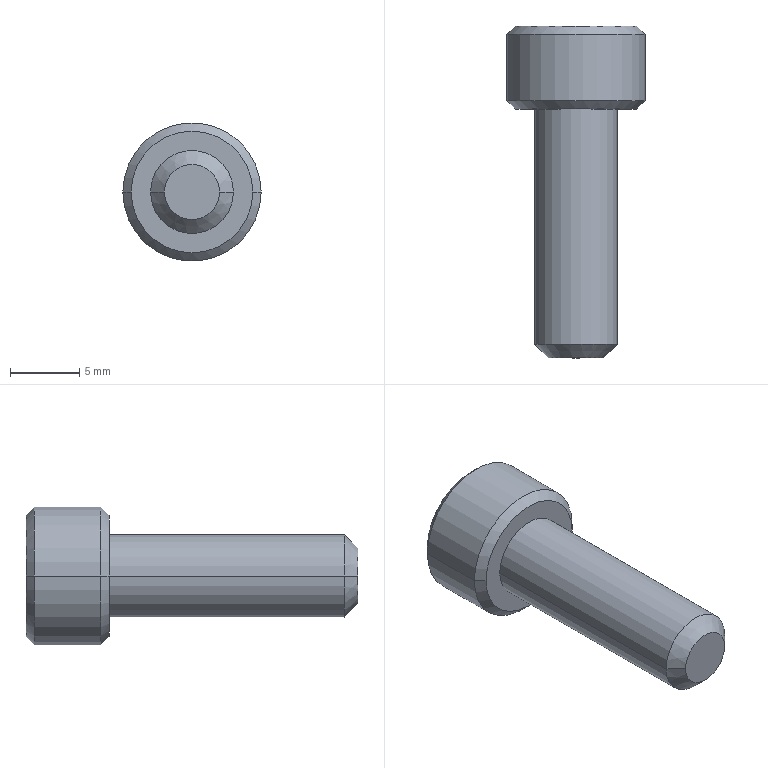Part | STEP file | BB62-M6-18L-6 | 1 solid | 27 faces | box 10 x 24 x 10 mm | volume 883.045 mm3 | plane 15 | cone 8 | cylinder 4 | commonest cylinder face diameters 6 x2 10 x2
STEP:
#1=CARTESIAN_POINT('',(0.,1.349,0.));
#2=VERTEX_POINT('',#1);
#3=CARTESIAN_POINT('',(2.86,3.,0.));
#4=VERTEX_POINT('',#3);
#5=CARTESIAN_POINT('',(0.,1.349,0.));
#6=DIRECTION('',(0.866,0.5,0.));
#7=VECTOR('',#6,1000.);
#8=LINE('',#5,#7);
#9=EDGE_CURVE('',#2,#4,#8,.T.);
#10=ORIENTED_EDGE('',*,*,#9,.F.);
#11=CARTESIAN_POINT('',(-2.86,3.,0.));
#12=VERTEX_POINT('',#11);
#13=CARTESIAN_POINT('',(0.,1.349,0.));
#14=DIRECTION('',(-0.866,0.5,0.));
#15=VECTOR('',#14,1000.);
#16=LINE('',#13,#15);
#17=EDGE_CURVE('',#2,#12,#16,.T.);
#18=ORIENTED_EDGE('',*,*,#17,.T.);
#19=CARTESIAN_POINT('',(-2.477,3.,1.43));
#20=VERTEX_POINT('',#19);
#21=CARTESIAN_POINT('',(0.,3.,0.));
#22=DIRECTION('',(0.,-1.,0.));
#23=DIRECTION('',(-1.,0.,0.));
#24=AXIS2_PLACEMENT_3D('',#21,#22,#23);
#25=CIRCLE('',#24,2.86);
#26=EDGE_CURVE('',#20,#12,#25,.T.);
#27=ORIENTED_EDGE('',*,*,#26,.F.);
#28=CARTESIAN_POINT('',(0.,3.,2.86));
#29=VERTEX_POINT('',#28);
#30=CARTESIAN_POINT('',(0.,3.,0.));
#31=DIRECTION('',(0.,-1.,0.));
#32=DIRECTION('',(-1.,0.,0.));
#33=AXIS2_PLACEMENT_3D('',#30,#31,#32);
#34=CIRCLE('',#33,2.86);
#35=EDGE_CURVE('',#29,#20,#34,.T.);
#36=ORIENTED_EDGE('',*,*,#35,.F.);
#37=CARTESIAN_POINT('',(2.477,3.,1.43));
#38=VERTEX_POINT('',#37);
#39=CARTESIAN_POINT('',(0.,3.,0.));
#40=DIRECTION('',(0.,-1.,0.));
#41=DIRECTION('',(-1.,0.,0.));
#42=AXIS2_PLACEMENT_3D('',#39,#40,#41);
#43=CIRCLE('',#42,2.86);
#44=EDGE_CURVE('',#38,#29,#43,.T.);
#45=ORIENTED_EDGE('',*,*,#44,.F.);
#46=CARTESIAN_POINT('',(0.,3.,0.));
#47=DIRECTION('',(0.,-1.,0.));
#48=DIRECTION('',(-1.,0.,0.));
#49=AXIS2_PLACEMENT_3D('',#46,#47,#48);
#50=CIRCLE('',#49,2.86);
#51=EDGE_CURVE('',#4,#38,#50,.T.);
#52=ORIENTED_EDGE('',*,*,#51,.F.);
#53=EDGE_LOOP('',(#10,#18,#27,#36,#45,#52));
#54=FACE_OUTER_BOUND('',#53,.T.);
#55=CARTESIAN_POINT('',(0.,1001.349,0.));
#56=DIRECTION('',(0.,1.,0.));
#57=DIRECTION('',(1.,0.,0.));
#58=AXIS2_PLACEMENT_3D('',#55,#56,#57);
#59=CONICAL_SURFACE('',#58,1732.051,1.047);
#60=ADVANCED_FACE('',(#54),#59,.F.);
#61=CARTESIAN_POINT('',(2.,-18.,0.));
#62=VERTEX_POINT('',#61);
#63=CARTESIAN_POINT('',(-2.,-18.,0.));
#64=VERTEX_POINT('',#63);
#65=CARTESIAN_POINT('',(0.,-18.,0.));
#66=DIRECTION('',(0.,1.,0.));
#67=DIRECTION('',(1.,0.,0.));
#68=AXIS2_PLACEMENT_3D('',#65,#66,#67);
#69=CIRCLE('',#68,2.);
#70=EDGE_CURVE('',#62,#64,#69,.T.);
#71=ORIENTED_EDGE('',*,*,#70,.T.);
#72=CARTESIAN_POINT('',(-3.,-17.,0.));
#73=VERTEX_POINT('',#72);
#74=CARTESIAN_POINT('',(-2.,-18.,0.));
#75=DIRECTION('',(-0.7071,0.7071,0.));
#76=VECTOR('',#75,1000.);
#77=LINE('',#74,#76);
#78=EDGE_CURVE('',#64,#73,#77,.T.);
#79=ORIENTED_EDGE('',*,*,#78,.T.);
#80=CARTESIAN_POINT('',(3.,-17.,0.));
#81=VERTEX_POINT('',#80);
#82=CARTESIAN_POINT('',(0.,-17.,0.));
#83=DIRECTION('',(0.,-1.,0.));
#84=DIRECTION('',(-1.,0.,0.));
#85=AXIS2_PLACEMENT_3D('',#82,#83,#84);
#86=CIRCLE('',#85,3.);
#87=EDGE_CURVE('',#73,#81,#86,.T.);
#88=ORIENTED_EDGE('',*,*,#87,.T.);
#89=CARTESIAN_POINT('',(2.,-18.,0.));
#90=DIRECTION('',(0.7071,0.7071,0.));
#91=VECTOR('',#90,1000.);
#92=LINE('',#89,#91);
#93=EDGE_CURVE('',#62,#81,#92,.T.);
#94=ORIENTED_EDGE('',*,*,#93,.F.);
#95=EDGE_LOOP('',(#71,#79,#88,#94));
#96=FACE_OUTER_BOUND('',#95,.T.);
#97=CARTESIAN_POINT('',(0.,-18.,0.));
#98=DIRECTION('',(0.,1.,0.));
#99=DIRECTION('',(1.,0.,0.));
#100=AXIS2_PLACEMENT_3D('',#97,#98,#99);
#101=CONICAL_SURFACE('',#100,2.,0.7854);
#102=ADVANCED_FACE('',(#96),#101,.T.);
#103=ORIENTED_EDGE('',*,*,#87,.F.);
#104=CARTESIAN_POINT('',(-3.,0.,0.));
#105=VERTEX_POINT('',#104);
#106=CARTESIAN_POINT('',(-3.,-17.,0.));
#107=DIRECTION('',(0.,1.,0.));
#108=VECTOR('',#107,1000.);
#109=LINE('',#106,#108);
#110=EDGE_CURVE('',#73,#105,#109,.T.);
#111=ORIENTED_EDGE('',*,*,#110,.T.);
#112=CARTESIAN_POINT('',(3.,0.,0.));
#113=VERTEX_POINT('',#112);
#114=CARTESIAN_POINT('',(0.,0.,0.));
#115=DIRECTION('',(0.,-1.,0.));
#116=DIRECTION('',(-1.,0.,0.));
#117=AXIS2_PLACEMENT_3D('',#114,#115,#116);
#118=CIRCLE('',#117,3.);
#119=EDGE_CURVE('',#105,#113,#118,.T.);
#120=ORIENTED_EDGE('',*,*,#119,.T.);
#121=CARTESIAN_POINT('',(3.,-17.,0.));
#122=DIRECTION('',(0.,1.,0.));
#123=VECTOR('',#122,1000.);
#124=LINE('',#121,#123);
#125=EDGE_CURVE('',#81,#113,#124,.T.);
#126=ORIENTED_EDGE('',*,*,#125,.F.);
#127=EDGE_LOOP('',(#103,#111,#120,#126));
#128=FACE_OUTER_BOUND('',#127,.T.);
#129=CARTESIAN_POINT('',(0.,-17.,0.));
#130=DIRECTION('',(0.,1.,0.));
#131=DIRECTION('',(1.,0.,0.));
#132=AXIS2_PLACEMENT_3D('',#129,#130,#131);
#133=CYLINDRICAL_SURFACE('',#132,3.);
#134=ADVANCED_FACE('',(#128),#133,.T.);
#135=CARTESIAN_POINT('',(-4.4,6.,0.));
#136=VERTEX_POINT('',#135);
#137=CARTESIAN_POINT('',(4.4,6.,0.));
#138=VERTEX_POINT('',#137);
#139=CARTESIAN_POINT('',(0.,6.,0.));
#140=DIRECTION('',(0.,-1.,0.));
#141=DIRECTION('',(-1.,0.,0.));
#142=AXIS2_PLACEMENT_3D('',#139,#140,#141);
#143=CIRCLE('',#142,4.4);
#144=EDGE_CURVE('',#136,#138,#143,.T.);
#145=ORIENTED_EDGE('',*,*,#144,.T.);
#146=CARTESIAN_POINT('',(5.,5.4,0.));
#147=VERTEX_POINT('',#146);
#148=CARTESIAN_POINT('',(5.,5.4,0.));
#149=DIRECTION('',(0.7071,-0.7071,0.));
#150=VECTOR('',#149,1000.);
#151=LINE('',#148,#150);
#152=EDGE_CURVE('',#138,#147,#151,.T.);
#153=ORIENTED_EDGE('',*,*,#152,.T.);
#154=CARTESIAN_POINT('',(-5.,5.4,0.));
#155=VERTEX_POINT('',#154);
#156=CARTESIAN_POINT('',(0.,5.4,0.));
#157=DIRECTION('',(0.,-1.,0.));
#158=DIRECTION('',(-1.,0.,0.));
#159=AXIS2_PLACEMENT_3D('',#156,#157,#158);
#160=CIRCLE('',#159,5.);
#161=EDGE_CURVE('',#155,#147,#160,.T.);
#162=ORIENTED_EDGE('',*,*,#161,.F.);
#163=CARTESIAN_POINT('',(-5.,5.4,0.));
#164=DIRECTION('',(-0.7071,-0.7071,0.));
#165=VECTOR('',#164,1000.);
#166=LINE('',#163,#165);
#167=EDGE_CURVE('',#136,#155,#166,.T.);
#168=ORIENTED_EDGE('',*,*,#167,.F.);
#169=EDGE_LOOP('',(#145,#153,#162,#168));
#170=FACE_OUTER_BOUND('',#169,.T.);
#171=CARTESIAN_POINT('',(0.,5.4,0.));
#172=DIRECTION('',(0.,-1.,0.));
#173=DIRECTION('',(-1.,0.,0.));
#174=AXIS2_PLACEMENT_3D('',#171,#172,#173);
#175=CONICAL_SURFACE('',#174,5.,0.7854);
#176=ADVANCED_FACE('',(#170),#175,.T.);
#177=ORIENTED_EDGE('',*,*,#161,.T.);
#178=CARTESIAN_POINT('',(5.,0.6,0.));
#179=VERTEX_POINT('',#178);
#180=CARTESIAN_POINT('',(5.,1.62,0.));
#181=DIRECTION('',(0.,-1.,0.));
#182=VECTOR('',#181,1000.);
#183=LINE('',#180,#182);
#184=EDGE_CURVE('',#147,#179,#183,.T.);
#185=ORIENTED_EDGE('',*,*,#184,.T.);
#186=CARTESIAN_POINT('',(-5.,0.6,0.));
#187=VERTEX_POINT('',#186);
#188=CARTESIAN_POINT('',(0.,0.6,0.));
#189=DIRECTION('',(0.,-1.,0.));
#190=DIRECTION('',(-1.,0.,0.));
#191=AXIS2_PLACEMENT_3D('',#188,#189,#190);
#192=CIRCLE('',#191,5.);
#193=EDGE_CURVE('',#187,#179,#192,.T.);
#194=ORIENTED_EDGE('',*,*,#193,.F.);
#195=CARTESIAN_POINT('',(-5.,1.62,0.));
#196=DIRECTION('',(0.,-1.,0.));
#197=VECTOR('',#196,1000.);
#198=LINE('',#195,#197);
#199=EDGE_CURVE('',#155,#187,#198,.T.);
#200=ORIENTED_EDGE('',*,*,#199,.F.);
#201=EDGE_LOOP('',(#177,#185,#194,#200));
#202=FACE_OUTER_BOUND('',#201,.T.);
#203=CARTESIAN_POINT('',(0.,1.62,0.));
#204=DIRECTION('',(0.,-1.,0.));
#205=DIRECTION('',(-1.,0.,0.));
#206=AXIS2_PLACEMENT_3D('',#203,#204,#205);
#207=CYLINDRICAL_SURFACE('',#206,5.);
#208=ADVANCED_FACE('',(#202),#207,.T.);
#209=CARTESIAN_POINT('',(-4.4,0.,0.));
#210=VERTEX_POINT('',#209);
#211=CARTESIAN_POINT('',(4.4,0.,0.));
#212=VERTEX_POINT('',#211);
#213=CARTESIAN_POINT('',(0.,0.,0.));
#214=DIRECTION('',(0.,-1.,0.));
#215=DIRECTION('',(-1.,0.,0.));
#216=AXIS2_PLACEMENT_3D('',#213,#214,#215);
#217=CIRCLE('',#216,4.4);
#218=EDGE_CURVE('',#210,#212,#217,.T.);
#219=ORIENTED_EDGE('',*,*,#218,.F.);
#220=CARTESIAN_POINT('',(-4.4,0.,0.));
#221=DIRECTION('',(-0.7071,0.7071,0.));
#222=VECTOR('',#221,1000.);
#223=LINE('',#220,#222);
#224=EDGE_CURVE('',#210,#187,#223,.T.);
#225=ORIENTED_EDGE('',*,*,#224,.T.);
#226=ORIENTED_EDGE('',*,*,#193,.T.);
#227=CARTESIAN_POINT('',(4.4,0.,0.));
#228=DIRECTION('',(0.7071,0.7071,0.));
#229=VECTOR('',#228,1000.);
#230=LINE('',#227,#229);
#231=EDGE_CURVE('',#212,#179,#230,.T.);
#232=ORIENTED_EDGE('',*,*,#231,.F.);
#233=EDGE_LOOP('',(#219,#225,#226,#232));
#234=FACE_OUTER_BOUND('',#233,.T.);
#235=CARTESIAN_POINT('',(0.,0.,0.));
#236=DIRECTION('',(0.,1.,0.));
#237=DIRECTION('',(1.,0.,0.));
#238=AXIS2_PLACEMENT_3D('',#235,#236,#237);
#239=CONICAL_SURFACE('',#238,4.4,0.7854);
#240=ADVANCED_FACE('',(#234),#239,.T.);
#241=ORIENTED_EDGE('',*,*,#144,.F.);
#242=CARTESIAN_POINT('',(0.,6.,0.));
#243=DIRECTION('',(0.,-1.,0.));
#244=DIRECTION('',(-1.,0.,0.));
#245=AXIS2_PLACEMENT_3D('',#242,#243,#244);
#246=CIRCLE('',#245,4.4);
#247=EDGE_CURVE('',#138,#136,#246,.T.);
#248=ORIENTED_EDGE('',*,*,#247,.F.);
#249=EDGE_LOOP('',(#241,#248));
#250=FACE_OUTER_BOUND('',#249,.T.);
#251=CARTESIAN_POINT('',(0.,6.,-2.86));
#252=VERTEX_POINT('',#251);
#253=CARTESIAN_POINT('',(-2.477,6.,-1.43));
#254=VERTEX_POINT('',#253);
#255=CARTESIAN_POINT('',(0.,6.,-2.86));
#256=DIRECTION('',(-0.866,0.,0.5));
#257=VECTOR('',#256,1000.);
#258=LINE('',#255,#257);
#259=EDGE_CURVE('',#252,#254,#258,.T.);
#260=ORIENTED_EDGE('',*,*,#259,.F.);
#261=CARTESIAN_POINT('',(2.477,6.,-1.43));
#262=VERTEX_POINT('',#261);
#263=CARTESIAN_POINT('',(2.477,6.,-1.43));
#264=DIRECTION('',(-0.866,0.,-0.5));
#265=VECTOR('',#264,1000.);
#266=LINE('',#263,#265);
#267=EDGE_CURVE('',#262,#252,#266,.T.);
#268=ORIENTED_EDGE('',*,*,#267,.F.);
#269=CARTESIAN_POINT('',(2.477,6.,1.43));
#270=VERTEX_POINT('',#269);
#271=CARTESIAN_POINT('',(2.477,6.,1.43));
#272=DIRECTION('',(0.,0.,-1.));
#273=VECTOR('',#272,1000.);
#274=LINE('',#271,#273);
#275=EDGE_CURVE('',#270,#262,#274,.T.);
#276=ORIENTED_EDGE('',*,*,#275,.F.);
#277=CARTESIAN_POINT('',(0.,6.,2.86));
#278=VERTEX_POINT('',#277);
#279=CARTESIAN_POINT('',(0.,6.,2.86));
#280=DIRECTION('',(0.866,0.,-0.5));
#281=VECTOR('',#280,1000.);
#282=LINE('',#279,#281);
#283=EDGE_CURVE('',#278,#270,#282,.T.);
#284=ORIENTED_EDGE('',*,*,#283,.F.);
#285=CARTESIAN_POINT('',(-2.477,6.,1.43));
#286=VERTEX_POINT('',#285);
#287=CARTESIAN_POINT('',(-2.477,6.,1.43));
#288=DIRECTION('',(0.866,0.,0.5));
#289=VECTOR('',#288,1000.);
#290=LINE('',#287,#289);
#291=EDGE_CURVE('',#286,#278,#290,.T.);
#292=ORIENTED_EDGE('',*,*,#291,.F.);
#293=CARTESIAN_POINT('',(-2.477,6.,-1.43));
#294=DIRECTION('',(0.,0.,1.));
#295=VECTOR('',#294,1000.);
#296=LINE('',#293,#295);
#297=EDGE_CURVE('',#254,#286,#296,.T.);
#298=ORIENTED_EDGE('',*,*,#297,.F.);
#299=EDGE_LOOP('',(#260,#268,#276,#284,#292,#298));
#300=FACE_BOUND('',#299,.T.);
#301=CARTESIAN_POINT('',(4.4,6.,0.));
#302=DIRECTION('',(0.,1.,0.));
#303=DIRECTION('',(1.,0.,0.));
#304=AXIS2_PLACEMENT_3D('',#301,#302,#303);
#305=PLANE('',#304);
#306=ADVANCED_FACE('',(#250,#300),#305,.T.);
#307=CARTESIAN_POINT('',(0.,0.,0.));
#308=DIRECTION('',(0.,-1.,0.));
#309=DIRECTION('',(-1.,0.,0.));
#310=AXIS2_PLACEMENT_3D('',#307,#308,#309);
#311=CIRCLE('',#310,3.);
#312=EDGE_CURVE('',#113,#105,#311,.T.);
#313=ORIENTED_EDGE('',*,*,#312,.F.);
#314=ORIENTED_EDGE('',*,*,#119,.F.);
#315=EDGE_LOOP('',(#313,#314));
#316=FACE_BOUND('',#315,.T.);
#317=CARTESIAN_POINT('',(0.,0.,0.));
#318=DIRECTION('',(0.,-1.,0.));
#319=DIRECTION('',(-1.,0.,0.));
#320=AXIS2_PLACEMENT_3D('',#317,#318,#319);
#321=CIRCLE('',#320,4.4);
#322=EDGE_CURVE('',#212,#210,#321,.T.);
#323=ORIENTED_EDGE('',*,*,#322,.T.);
#324=ORIENTED_EDGE('',*,*,#218,.T.);
#325=EDGE_LOOP('',(#323,#324));
#326=FACE_OUTER_BOUND('',#325,.T.);
#327=CARTESIAN_POINT('',(0.,0.,0.));
#328=DIRECTION('',(0.,-1.,0.));
#329=DIRECTION('',(-1.,0.,0.));
#330=AXIS2_PLACEMENT_3D('',#327,#328,#329);
#331=PLANE('',#330);
#332=ADVANCED_FACE('',(#316,#326),#331,.T.);
#333=ORIENTED_EDGE('',*,*,#224,.F.);
#334=ORIENTED_EDGE('',*,*,#322,.F.);
#335=ORIENTED_EDGE('',*,*,#231,.T.);
#336=CARTESIAN_POINT('',(0.,0.6,0.));
#337=DIRECTION('',(0.,-1.,0.));
#338=DIRECTION('',(-1.,0.,0.));
#339=AXIS2_PLACEMENT_3D('',#336,#337,#338);
#340=CIRCLE('',#339,5.);
#341=EDGE_CURVE('',#179,#187,#340,.T.);
#342=ORIENTED_EDGE('',*,*,#341,.T.);
#343=EDGE_LOOP('',(#333,#334,#335,#342));
#344=FACE_OUTER_BOUND('',#343,.T.);
#345=CARTESIAN_POINT('',(0.,0.,0.));
#346=DIRECTION('',(0.,1.,0.));
#347=DIRECTION('',(1.,0.,0.));
#348=AXIS2_PLACEMENT_3D('',#345,#346,#347);
#349=CONICAL_SURFACE('',#348,4.4,0.7854);
#350=ADVANCED_FACE('',(#344),#349,.T.);
#351=ORIENTED_EDGE('',*,*,#184,.F.);
#352=CARTESIAN_POINT('',(0.,5.4,0.));
#353=DIRECTION('',(0.,-1.,0.));
#354=DIRECTION('',(-1.,0.,0.));
#355=AXIS2_PLACEMENT_3D('',#352,#353,#354);
#356=CIRCLE('',#355,5.);
#357=EDGE_CURVE('',#147,#155,#356,.T.);
#358=ORIENTED_EDGE('',*,*,#357,.T.);
#359=ORIENTED_EDGE('',*,*,#199,.T.);
#360=ORIENTED_EDGE('',*,*,#341,.F.);
#361=EDGE_LOOP('',(#351,#358,#359,#360));
#362=FACE_OUTER_BOUND('',#361,.T.);
#363=CARTESIAN_POINT('',(0.,1.62,0.));
#364=DIRECTION('',(0.,-1.,0.));
#365=DIRECTION('',(-1.,0.,0.));
#366=AXIS2_PLACEMENT_3D('',#363,#364,#365);
#367=CYLINDRICAL_SURFACE('',#366,5.);
#368=ADVANCED_FACE('',(#362),#367,.T.);
#369=ORIENTED_EDGE('',*,*,#152,.F.);
#370=ORIENTED_EDGE('',*,*,#247,.T.);
#371=ORIENTED_EDGE('',*,*,#167,.T.);
#372=ORIENTED_EDGE('',*,*,#357,.F.);
#373=EDGE_LOOP('',(#369,#370,#371,#372));
#374=FACE_OUTER_BOUND('',#373,.T.);
#375=CARTESIAN_POINT('',(0.,5.4,0.));
#376=DIRECTION('',(0.,-1.,0.));
#377=DIRECTION('',(-1.,0.,0.));
#378=AXIS2_PLACEMENT_3D('',#375,#376,#377);
#379=CONICAL_SURFACE('',#378,5.,0.7854);
#380=ADVANCED_FACE('',(#374),#379,.T.);
#381=ORIENTED_EDGE('',*,*,#110,.F.);
#382=CARTESIAN_POINT('',(0.,-17.,0.));
#383=DIRECTION('',(0.,-1.,0.));
#384=DIRECTION('',(-1.,0.,0.));
#385=AXIS2_PLACEMENT_3D('',#382,#383,#384);
#386=CIRCLE('',#385,3.);
#387=EDGE_CURVE('',#81,#73,#386,.T.);
#388=ORIENTED_EDGE('',*,*,#387,.F.);
#389=ORIENTED_EDGE('',*,*,#125,.T.);
#390=ORIENTED_EDGE('',*,*,#312,.T.);
#391=EDGE_LOOP('',(#381,#388,#389,#390));
#392=FACE_OUTER_BOUND('',#391,.T.);
#393=CARTESIAN_POINT('',(0.,-17.,0.));
#394=DIRECTION('',(0.,1.,0.));
#395=DIRECTION('',(1.,0.,0.));
#396=AXIS2_PLACEMENT_3D('',#393,#394,#395);
#397=CYLINDRICAL_SURFACE('',#396,3.);
#398=ADVANCED_FACE('',(#392),#397,.T.);
#399=ORIENTED_EDGE('',*,*,#70,.F.);
#400=CARTESIAN_POINT('',(0.,-18.,0.));
#401=DIRECTION('',(0.,1.,0.));
#402=DIRECTION('',(1.,0.,0.));
#403=AXIS2_PLACEMENT_3D('',#400,#401,#402);
#404=CIRCLE('',#403,2.);
#405=EDGE_CURVE('',#64,#62,#404,.T.);
#406=ORIENTED_EDGE('',*,*,#405,.F.);
#407=EDGE_LOOP('',(#399,#406));
#408=FACE_OUTER_BOUND('',#407,.T.);
#409=CARTESIAN_POINT('',(0.,-18.,0.));
#410=DIRECTION('',(0.,-1.,0.));
#411=DIRECTION('',(-1.,0.,0.));
#412=AXIS2_PLACEMENT_3D('',#409,#410,#411);
#413=PLANE('',#412);
#414=ADVANCED_FACE('',(#408),#413,.T.);
#415=ORIENTED_EDGE('',*,*,#78,.F.);
#416=ORIENTED_EDGE('',*,*,#405,.T.);
#417=ORIENTED_EDGE('',*,*,#93,.T.);
#418=ORIENTED_EDGE('',*,*,#387,.T.);
#419=EDGE_LOOP('',(#415,#416,#417,#418));
#420=FACE_OUTER_BOUND('',#419,.T.);
#421=CARTESIAN_POINT('',(0.,-18.,0.));
#422=DIRECTION('',(0.,1.,0.));
#423=DIRECTION('',(1.,0.,0.));
#424=AXIS2_PLACEMENT_3D('',#421,#422,#423);
#425=CONICAL_SURFACE('',#424,2.,0.7854);
#426=ADVANCED_FACE('',(#420),#425,.T.);
#427=CARTESIAN_POINT('',(2.477,3.,-1.43));
#428=VERTEX_POINT('',#427);
#429=CARTESIAN_POINT('',(0.,3.,-2.86));
#430=VERTEX_POINT('',#429);
#431=CARTESIAN_POINT('',(2.477,3.,-1.43));
#432=DIRECTION('',(-0.866,0.,-0.5));
#433=VECTOR('',#432,1000.);
#434=LINE('',#431,#433);
#435=EDGE_CURVE('',#428,#430,#434,.T.);
#436=ORIENTED_EDGE('',*,*,#435,.F.);
#437=CARTESIAN_POINT('',(2.477,6.,-1.43));
#438=DIRECTION('',(0.,-1.,0.));
#439=VECTOR('',#438,1000.);
#440=LINE('',#437,#439);
#441=EDGE_CURVE('',#262,#428,#440,.T.);
#442=ORIENTED_EDGE('',*,*,#441,.F.);
#443=ORIENTED_EDGE('',*,*,#267,.T.);
#444=CARTESIAN_POINT('',(0.,6.,-2.86));
#445=DIRECTION('',(0.,-1.,0.));
#446=VECTOR('',#445,1000.);
#447=LINE('',#444,#446);
#448=EDGE_CURVE('',#252,#430,#447,.T.);
#449=ORIENTED_EDGE('',*,*,#448,.T.);
#450=EDGE_LOOP('',(#436,#442,#443,#449));
#451=FACE_OUTER_BOUND('',#450,.T.);
#452=CARTESIAN_POINT('',(2.477,6.,-1.43));
#453=DIRECTION('',(-0.5,0.,0.866));
#454=DIRECTION('',(0.866,0.,0.5));
#455=AXIS2_PLACEMENT_3D('',#452,#453,#454);
#456=PLANE('',#455);
#457=ADVANCED_FACE('',(#451),#456,.T.);
#458=CARTESIAN_POINT('',(-2.477,3.,-1.43));
#459=VERTEX_POINT('',#458);
#460=CARTESIAN_POINT('',(0.,3.,-2.86));
#461=DIRECTION('',(-0.866,0.,0.5));
#462=VECTOR('',#461,1000.);
#463=LINE('',#460,#462);
#464=EDGE_CURVE('',#430,#459,#463,.T.);
#465=ORIENTED_EDGE('',*,*,#464,.F.);
#466=ORIENTED_EDGE('',*,*,#448,.F.);
#467=ORIENTED_EDGE('',*,*,#259,.T.);
#468=CARTESIAN_POINT('',(-2.477,6.,-1.43));
#469=DIRECTION('',(0.,-1.,0.));
#470=VECTOR('',#469,1000.);
#471=LINE('',#468,#470);
#472=EDGE_CURVE('',#254,#459,#471,.T.);
#473=ORIENTED_EDGE('',*,*,#472,.T.);
#474=EDGE_LOOP('',(#465,#466,#467,#473));
#475=FACE_OUTER_BOUND('',#474,.T.);
#476=CARTESIAN_POINT('',(0.,6.,-2.86));
#477=DIRECTION('',(0.5,0.,0.866));
#478=DIRECTION('',(0.866,0.,-0.5));
#479=AXIS2_PLACEMENT_3D('',#476,#477,#478);
#480=PLANE('',#479);
#481=ADVANCED_FACE('',(#475),#480,.T.);
#482=CARTESIAN_POINT('',(-2.477,3.,-1.43));
#483=DIRECTION('',(0.,0.,1.));
#484=VECTOR('',#483,1000.);
#485=LINE('',#482,#484);
#486=EDGE_CURVE('',#459,#20,#485,.T.);
#487=ORIENTED_EDGE('',*,*,#486,.F.);
#488=ORIENTED_EDGE('',*,*,#472,.F.);
#489=ORIENTED_EDGE('',*,*,#297,.T.);
#490=CARTESIAN_POINT('',(-2.477,6.,1.43));
#491=DIRECTION('',(0.,-1.,0.));
#492=VECTOR('',#491,1000.);
#493=LINE('',#490,#492);
#494=EDGE_CURVE('',#286,#20,#493,.T.);
#495=ORIENTED_EDGE('',*,*,#494,.T.);
#496=EDGE_LOOP('',(#487,#488,#489,#495));
#497=FACE_OUTER_BOUND('',#496,.T.);
#498=CARTESIAN_POINT('',(-2.477,6.,-1.43));
#499=DIRECTION('',(1.,0.,0.));
#500=DIRECTION('',(0.,0.,-1.));
#501=AXIS2_PLACEMENT_3D('',#498,#499,#500);
#502=PLANE('',#501);
#503=ADVANCED_FACE('',(#497),#502,.T.);
#504=CARTESIAN_POINT('',(-2.477,3.,1.43));
#505=DIRECTION('',(0.866,0.,0.5));
#506=VECTOR('',#505,1000.);
#507=LINE('',#504,#506);
#508=EDGE_CURVE('',#20,#29,#507,.T.);
#509=ORIENTED_EDGE('',*,*,#508,.F.);
#510=ORIENTED_EDGE('',*,*,#494,.F.);
#511=ORIENTED_EDGE('',*,*,#291,.T.);
#512=CARTESIAN_POINT('',(0.,6.,2.86));
#513=DIRECTION('',(0.,-1.,0.));
#514=VECTOR('',#513,1000.);
#515=LINE('',#512,#514);
#516=EDGE_CURVE('',#278,#29,#515,.T.);
#517=ORIENTED_EDGE('',*,*,#516,.T.);
#518=EDGE_LOOP('',(#509,#510,#511,#517));
#519=FACE_OUTER_BOUND('',#518,.T.);
#520=CARTESIAN_POINT('',(-2.477,6.,1.43));
#521=DIRECTION('',(0.5,0.,-0.866));
#522=DIRECTION('',(-0.866,0.,-0.5));
#523=AXIS2_PLACEMENT_3D('',#520,#521,#522);
#524=PLANE('',#523);
#525=ADVANCED_FACE('',(#519),#524,.T.);
#526=CARTESIAN_POINT('',(0.,3.,2.86));
#527=DIRECTION('',(0.866,0.,-0.5));
#528=VECTOR('',#527,1000.);
#529=LINE('',#526,#528);
#530=EDGE_CURVE('',#29,#38,#529,.T.);
#531=ORIENTED_EDGE('',*,*,#530,.F.);
#532=ORIENTED_EDGE('',*,*,#516,.F.);
#533=ORIENTED_EDGE('',*,*,#283,.T.);
#534=CARTESIAN_POINT('',(2.477,6.,1.43));
#535=DIRECTION('',(0.,-1.,0.));
#536=VECTOR('',#535,1000.);
#537=LINE('',#534,#536);
#538=EDGE_CURVE('',#270,#38,#537,.T.);
#539=ORIENTED_EDGE('',*,*,#538,.T.);
#540=EDGE_LOOP('',(#531,#532,#533,#539));
#541=FACE_OUTER_BOUND('',#540,.T.);
#542=CARTESIAN_POINT('',(0.,6.,2.86));
#543=DIRECTION('',(-0.5,0.,-0.866));
#544=DIRECTION('',(-0.866,0.,0.5));
#545=AXIS2_PLACEMENT_3D('',#542,#543,#544);
#546=PLANE('',#545);
#547=ADVANCED_FACE('',(#541),#546,.T.);
#548=CARTESIAN_POINT('',(2.477,3.,1.43));
#549=DIRECTION('',(0.,0.,-1.));
#550=VECTOR('',#549,1000.);
#551=LINE('',#548,#550);
#552=EDGE_CURVE('',#38,#428,#551,.T.);
#553=ORIENTED_EDGE('',*,*,#552,.F.);
#554=ORIENTED_EDGE('',*,*,#538,.F.);
#555=ORIENTED_EDGE('',*,*,#275,.T.);
#556=ORIENTED_EDGE('',*,*,#441,.T.);
#557=EDGE_LOOP('',(#553,#554,#555,#556));
#558=FACE_OUTER_BOUND('',#557,.T.);
#559=CARTESIAN_POINT('',(2.477,6.,1.43));
#560=DIRECTION('',(-1.,0.,0.));
#561=DIRECTION('',(0.,0.,1.));
#562=AXIS2_PLACEMENT_3D('',#559,#560,#561);
#563=PLANE('',#562);
#564=ADVANCED_FACE('',(#558),#563,.T.);
#565=ORIENTED_EDGE('',*,*,#435,.T.);
#566=CARTESIAN_POINT('',(0.,3.,0.));
#567=DIRECTION('',(0.,-1.,0.));
#568=DIRECTION('',(-1.,0.,0.));
#569=AXIS2_PLACEMENT_3D('',#566,#567,#568);
#570=CIRCLE('',#569,2.86);
#571=EDGE_CURVE('',#430,#428,#570,.T.);
#572=ORIENTED_EDGE('',*,*,#571,.T.);
#573=EDGE_LOOP('',(#565,#572));
#574=FACE_OUTER_BOUND('',#573,.T.);
#575=CARTESIAN_POINT('',(0.,3.,0.));
#576=DIRECTION('',(0.,1.,0.));
#577=DIRECTION('',(1.,0.,0.));
#578=AXIS2_PLACEMENT_3D('',#575,#576,#577);
#579=PLANE('',#578);
#580=ADVANCED_FACE('',(#574),#579,.F.);
#581=ORIENTED_EDGE('',*,*,#552,.T.);
#582=CARTESIAN_POINT('',(0.,3.,0.));
#583=DIRECTION('',(0.,-1.,0.));
#584=DIRECTION('',(-1.,0.,0.));
#585=AXIS2_PLACEMENT_3D('',#582,#583,#584);
#586=CIRCLE('',#585,2.86);
#587=EDGE_CURVE('',#428,#4,#586,.T.);
#588=ORIENTED_EDGE('',*,*,#587,.T.);
#589=ORIENTED_EDGE('',*,*,#51,.T.);
#590=EDGE_LOOP('',(#581,#588,#589));
#591=FACE_OUTER_BOUND('',#590,.T.);
#592=CARTESIAN_POINT('',(0.,3.,0.));
#593=DIRECTION('',(0.,1.,0.));
#594=DIRECTION('',(1.,0.,0.));
#595=AXIS2_PLACEMENT_3D('',#592,#593,#594);
#596=PLANE('',#595);
#597=ADVANCED_FACE('',(#591),#596,.F.);
#598=ORIENTED_EDGE('',*,*,#530,.T.);
#599=ORIENTED_EDGE('',*,*,#44,.T.);
#600=EDGE_LOOP('',(#598,#599));
#601=FACE_OUTER_BOUND('',#600,.T.);
#602=CARTESIAN_POINT('',(0.,3.,0.));
#603=DIRECTION('',(0.,1.,0.));
#604=DIRECTION('',(1.,0.,0.));
#605=AXIS2_PLACEMENT_3D('',#602,#603,#604);
#606=PLANE('',#605);
#607=ADVANCED_FACE('',(#601),#606,.F.);
#608=ORIENTED_EDGE('',*,*,#508,.T.);
#609=ORIENTED_EDGE('',*,*,#35,.T.);
#610=EDGE_LOOP('',(#608,#609));
#611=FACE_OUTER_BOUND('',#610,.T.);
#612=CARTESIAN_POINT('',(0.,3.,0.));
#613=DIRECTION('',(0.,1.,0.));
#614=DIRECTION('',(1.,0.,0.));
#615=AXIS2_PLACEMENT_3D('',#612,#613,#614);
#616=PLANE('',#615);
#617=ADVANCED_FACE('',(#611),#616,.F.);
#618=ORIENTED_EDGE('',*,*,#486,.T.);
#619=ORIENTED_EDGE('',*,*,#26,.T.);
#620=CARTESIAN_POINT('',(0.,3.,0.));
#621=DIRECTION('',(0.,-1.,0.));
#622=DIRECTION('',(-1.,0.,0.));
#623=AXIS2_PLACEMENT_3D('',#620,#621,#622);
#624=CIRCLE('',#623,2.86);
#625=EDGE_CURVE('',#12,#459,#624,.T.);
#626=ORIENTED_EDGE('',*,*,#625,.T.);
#627=EDGE_LOOP('',(#618,#619,#626));
#628=FACE_OUTER_BOUND('',#627,.T.);
#629=CARTESIAN_POINT('',(0.,3.,0.));
#630=DIRECTION('',(0.,1.,0.));
#631=DIRECTION('',(1.,0.,0.));
#632=AXIS2_PLACEMENT_3D('',#629,#630,#631);
#633=PLANE('',#632);
#634=ADVANCED_FACE('',(#628),#633,.F.);
#635=ORIENTED_EDGE('',*,*,#464,.T.);
#636=CARTESIAN_POINT('',(0.,3.,0.));
#637=DIRECTION('',(0.,-1.,0.));
#638=DIRECTION('',(-1.,0.,0.));
#639=AXIS2_PLACEMENT_3D('',#636,#637,#638);
#640=CIRCLE('',#639,2.86);
#641=EDGE_CURVE('',#459,#430,#640,.T.);
#642=ORIENTED_EDGE('',*,*,#641,.T.);
#643=EDGE_LOOP('',(#635,#642));
#644=FACE_OUTER_BOUND('',#643,.T.);
#645=CARTESIAN_POINT('',(0.,3.,0.));
#646=DIRECTION('',(0.,1.,0.));
#647=DIRECTION('',(1.,0.,0.));
#648=AXIS2_PLACEMENT_3D('',#645,#646,#647);
#649=PLANE('',#648);
#650=ADVANCED_FACE('',(#644),#649,.F.);
#651=ORIENTED_EDGE('',*,*,#17,.F.);
#652=ORIENTED_EDGE('',*,*,#9,.T.);
#653=ORIENTED_EDGE('',*,*,#587,.F.);
#654=ORIENTED_EDGE('',*,*,#571,.F.);
#655=ORIENTED_EDGE('',*,*,#641,.F.);
#656=ORIENTED_EDGE('',*,*,#625,.F.);
#657=EDGE_LOOP('',(#651,#652,#653,#654,#655,#656));
#658=FACE_OUTER_BOUND('',#657,.T.);
#659=CARTESIAN_POINT('',(0.,1001.349,0.));
#660=DIRECTION('',(0.,1.,0.));
#661=DIRECTION('',(1.,0.,0.));
#662=AXIS2_PLACEMENT_3D('',#659,#660,#661);
#663=CONICAL_SURFACE('',#662,1732.051,1.047);
#664=ADVANCED_FACE('',(#658),#663,.F.);
#665=CLOSED_SHELL('',(#60,#102,#134,#176,#208,#240,#306,#332,#350,#368,#380,#398,#414,#426,#457,#481,#503,#525,#547,#564,#580,#597,#607,#617,#634,#650,#664));
#666=MANIFOLD_SOLID_BREP('',#665);
#667=CARTESIAN_POINT('',(0.,0.,0.));
#668=DIRECTION('',(0.,0.,1.));
#669=DIRECTION('',(1.,0.,0.));
#670=AXIS2_PLACEMENT_3D('',#667,#668,#669);
#671=(LENGTH_UNIT()NAMED_UNIT(*)SI_UNIT(.MILLI.,.METRE.));
#672=UNCERTAINTY_MEASURE_WITH_UNIT(LENGTH_MEASURE(0.00001),#671,'','');
#673=(NAMED_UNIT(*)PLANE_ANGLE_UNIT()SI_UNIT($,.RADIAN.));
#674=(NAMED_UNIT(*)SI_UNIT($,.STERADIAN.)SOLID_ANGLE_UNIT());
#675=(GEOMETRIC_REPRESENTATION_CONTEXT(3)GLOBAL_UNCERTAINTY_ASSIGNED_CONTEXT((#672))GLOBAL_UNIT_ASSIGNED_CONTEXT((#671,#673,#674))REPRESENTATION_CONTEXT('',''));
#676=ADVANCED_BREP_SHAPE_REPRESENTATION('',(#666,#670),#675);